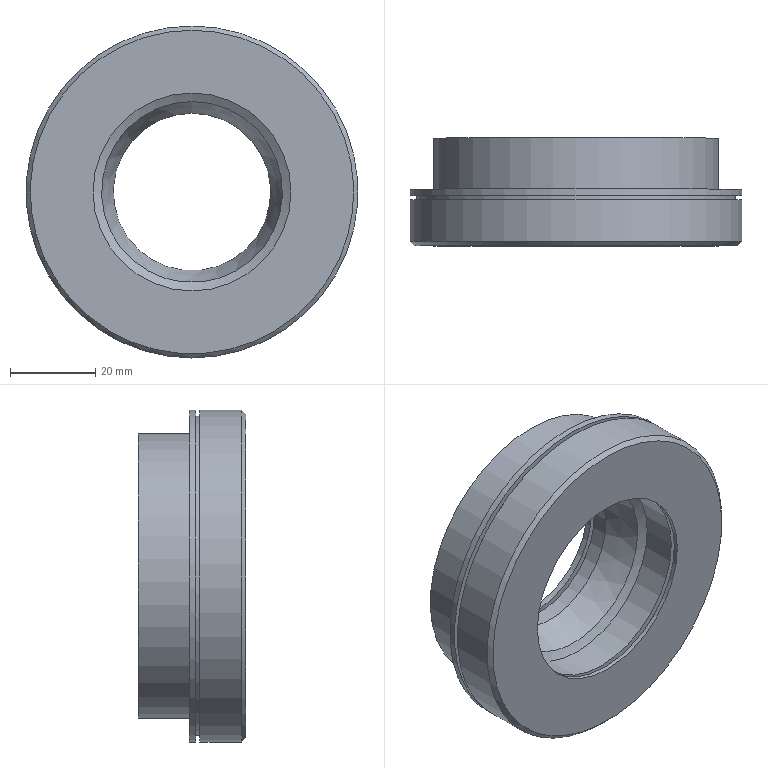Part | STEP file | Inner part of clamp | 1 solid | 38 faces | box 78 x 25.32 x 78 mm | volume 67715 mm3 | cylinder 14 | plane 13 | cone 7 | torus 4 | commonest cylinder face diameters 8 x4 37 x2 46.5 x2 78 x2 40 x1 49.5 x1
STEP:
#1=CARTESIAN_POINT('',(0.,-14.5,39.));
#2=VERTEX_POINT('',#1);
#3=CARTESIAN_POINT('',(0.,-14.5,0.));
#4=DIRECTION('',(0.,1.,0.));
#5=DIRECTION('',(0.,0.,1.));
#6=AXIS2_PLACEMENT_3D('',#3,#4,#5);
#7=CIRCLE('',#6,39.);
#8=EDGE_CURVE('',#2,#2,#7,.F.);
#9=ORIENTED_EDGE('',*,*,#8,.T.);
#10=EDGE_LOOP('',(#9));
#11=FACE_OUTER_BOUND('',#10,.T.);
#12=CARTESIAN_POINT('',(0.,-24.32,39.));
#13=VERTEX_POINT('',#12);
#14=CARTESIAN_POINT('',(0.,-24.32,0.));
#15=DIRECTION('',(0.,1.,0.));
#16=DIRECTION('',(0.,0.,1.));
#17=AXIS2_PLACEMENT_3D('',#14,#15,#16);
#18=CIRCLE('',#17,39.);
#19=EDGE_CURVE('',#13,#13,#18,.T.);
#20=ORIENTED_EDGE('',*,*,#19,.T.);
#21=EDGE_LOOP('',(#20));
#22=FACE_OUTER_BOUND('',#21,.T.);
#23=CARTESIAN_POINT('',(0.,-22.,0.));
#24=DIRECTION('',(0.,1.,0.));
#25=DIRECTION('',(0.,0.,1.));
#26=AXIS2_PLACEMENT_3D('',#23,#24,#25);
#27=CYLINDRICAL_SURFACE('',#26,39.);
#28=ADVANCED_FACE('',(#11,#22),#27,.T.);
#29=CARTESIAN_POINT('',(0.,-25.32,38.));
#30=VERTEX_POINT('',#29);
#31=CARTESIAN_POINT('',(0.,-25.32,0.));
#32=DIRECTION('',(0.,1.,0.));
#33=DIRECTION('',(0.,0.,1.));
#34=AXIS2_PLACEMENT_3D('',#31,#32,#33);
#35=CIRCLE('',#34,38.);
#36=EDGE_CURVE('',#30,#30,#35,.T.);
#37=ORIENTED_EDGE('',*,*,#36,.F.);
#38=EDGE_LOOP('',(#37));
#39=FACE_BOUND('',#38,.T.);
#40=CARTESIAN_POINT('',(0.,-25.32,23.25));
#41=VERTEX_POINT('',#40);
#42=CARTESIAN_POINT('',(0.,-25.32,0.));
#43=DIRECTION('',(0.,1.,0.));
#44=DIRECTION('',(0.,0.,1.));
#45=AXIS2_PLACEMENT_3D('',#42,#43,#44);
#46=CIRCLE('',#45,23.25);
#47=EDGE_CURVE('',#41,#41,#46,.T.);
#48=ORIENTED_EDGE('',*,*,#47,.T.);
#49=EDGE_LOOP('',(#48));
#50=FACE_BOUND('',#49,.T.);
#51=CARTESIAN_POINT('',(0.,-25.32,0.));
#52=DIRECTION('',(0.,-1.,0.));
#53=DIRECTION('',(0.,0.,1.));
#54=AXIS2_PLACEMENT_3D('',#51,#52,#53);
#55=PLANE('',#54);
#56=ADVANCED_FACE('',(#39,#50),#55,.T.);
#57=ORIENTED_EDGE('',*,*,#8,.F.);
#58=EDGE_LOOP('',(#57));
#59=FACE_BOUND('',#58,.T.);
#60=CARTESIAN_POINT('',(0.,-14.5,37.5));
#61=VERTEX_POINT('',#60);
#62=CARTESIAN_POINT('',(0.,-14.5,0.));
#63=DIRECTION('',(0.,1.,0.));
#64=DIRECTION('',(0.,0.,1.));
#65=AXIS2_PLACEMENT_3D('',#62,#63,#64);
#66=CIRCLE('',#65,37.5);
#67=EDGE_CURVE('',#61,#61,#66,.T.);
#68=ORIENTED_EDGE('',*,*,#67,.F.);
#69=EDGE_LOOP('',(#68));
#70=FACE_BOUND('',#69,.T.);
#71=CARTESIAN_POINT('',(0.,-14.5,0.));
#72=DIRECTION('',(0.,-1.,0.));
#73=DIRECTION('',(0.,0.,1.));
#74=AXIS2_PLACEMENT_3D('',#71,#72,#73);
#75=PLANE('',#74);
#76=ADVANCED_FACE('',(#59,#70),#75,.F.);
#77=CARTESIAN_POINT('',(0.,-24.32,23.25));
#78=VERTEX_POINT('',#77);
#79=CARTESIAN_POINT('',(0.,-24.32,0.));
#80=DIRECTION('',(0.,1.,0.));
#81=DIRECTION('',(0.,0.,1.));
#82=AXIS2_PLACEMENT_3D('',#79,#80,#81);
#83=CIRCLE('',#82,23.25);
#84=EDGE_CURVE('',#78,#78,#83,.T.);
#85=ORIENTED_EDGE('',*,*,#84,.T.);
#86=EDGE_LOOP('',(#85));
#87=FACE_OUTER_BOUND('',#86,.T.);
#88=ORIENTED_EDGE('',*,*,#47,.F.);
#89=EDGE_LOOP('',(#88));
#90=FACE_OUTER_BOUND('',#89,.T.);
#91=CARTESIAN_POINT('',(0.,-15.32,0.));
#92=DIRECTION('',(0.,1.,0.));
#93=DIRECTION('',(0.,0.,1.));
#94=AXIS2_PLACEMENT_3D('',#91,#92,#93);
#95=CYLINDRICAL_SURFACE('',#94,23.25);
#96=ADVANCED_FACE('',(#87,#90),#95,.F.);
#97=CARTESIAN_POINT('',(0.,-13.5,37.5));
#98=VERTEX_POINT('',#97);
#99=CARTESIAN_POINT('',(0.,-13.5,0.));
#100=DIRECTION('',(0.,1.,0.));
#101=DIRECTION('',(0.,0.,1.));
#102=AXIS2_PLACEMENT_3D('',#99,#100,#101);
#103=CIRCLE('',#102,37.5);
#104=EDGE_CURVE('',#98,#98,#103,.T.);
#105=ORIENTED_EDGE('',*,*,#104,.F.);
#106=EDGE_LOOP('',(#105));
#107=FACE_OUTER_BOUND('',#106,.T.);
#108=ORIENTED_EDGE('',*,*,#67,.T.);
#109=EDGE_LOOP('',(#108));
#110=FACE_OUTER_BOUND('',#109,.T.);
#111=CARTESIAN_POINT('',(0.,-13.5,0.));
#112=DIRECTION('',(0.,1.,0.));
#113=DIRECTION('',(0.,0.,1.));
#114=AXIS2_PLACEMENT_3D('',#111,#112,#113);
#115=CYLINDRICAL_SURFACE('',#114,37.5);
#116=ADVANCED_FACE('',(#107,#110),#115,.T.);
#117=CARTESIAN_POINT('',(0.,-24.32,24.75));
#118=VERTEX_POINT('',#117);
#119=CARTESIAN_POINT('',(0.,-24.32,0.));
#120=DIRECTION('',(0.,1.,0.));
#121=DIRECTION('',(0.,0.,1.));
#122=AXIS2_PLACEMENT_3D('',#119,#120,#121);
#123=CIRCLE('',#122,24.75);
#124=EDGE_CURVE('',#118,#118,#123,.T.);
#125=ORIENTED_EDGE('',*,*,#124,.T.);
#126=EDGE_LOOP('',(#125));
#127=FACE_BOUND('',#126,.T.);
#128=ORIENTED_EDGE('',*,*,#84,.F.);
#129=EDGE_LOOP('',(#128));
#130=FACE_BOUND('',#129,.T.);
#131=CARTESIAN_POINT('',(0.,-24.32,0.));
#132=DIRECTION('',(0.,-1.,0.));
#133=DIRECTION('',(0.,0.,1.));
#134=AXIS2_PLACEMENT_3D('',#131,#132,#133);
#135=PLANE('',#134);
#136=ADVANCED_FACE('',(#127,#130),#135,.F.);
#137=CARTESIAN_POINT('',(0.,-13.5,39.));
#138=VERTEX_POINT('',#137);
#139=CARTESIAN_POINT('',(0.,-13.5,0.));
#140=DIRECTION('',(0.,1.,0.));
#141=DIRECTION('',(0.,0.,1.));
#142=AXIS2_PLACEMENT_3D('',#139,#140,#141);
#143=CIRCLE('',#142,39.);
#144=EDGE_CURVE('',#138,#138,#143,.T.);
#145=ORIENTED_EDGE('',*,*,#144,.F.);
#146=EDGE_LOOP('',(#145));
#147=FACE_BOUND('',#146,.T.);
#148=ORIENTED_EDGE('',*,*,#104,.T.);
#149=EDGE_LOOP('',(#148));
#150=FACE_BOUND('',#149,.T.);
#151=CARTESIAN_POINT('',(0.,-13.5,0.));
#152=DIRECTION('',(0.,1.,0.));
#153=DIRECTION('',(0.,0.,1.));
#154=AXIS2_PLACEMENT_3D('',#151,#152,#153);
#155=PLANE('',#154);
#156=ADVANCED_FACE('',(#147,#150),#155,.F.);
#157=CARTESIAN_POINT('',(0.,-23.32,24.75));
#158=VERTEX_POINT('',#157);
#159=CARTESIAN_POINT('',(0.,-23.32,0.));
#160=DIRECTION('',(0.,1.,0.));
#161=DIRECTION('',(0.,0.,1.));
#162=AXIS2_PLACEMENT_3D('',#159,#160,#161);
#163=CIRCLE('',#162,24.75);
#164=EDGE_CURVE('',#158,#158,#163,.T.);
#165=ORIENTED_EDGE('',*,*,#164,.T.);
#166=EDGE_LOOP('',(#165));
#167=FACE_OUTER_BOUND('',#166,.T.);
#168=ORIENTED_EDGE('',*,*,#124,.F.);
#169=EDGE_LOOP('',(#168));
#170=FACE_OUTER_BOUND('',#169,.T.);
#171=CARTESIAN_POINT('',(0.,-24.32,0.));
#172=DIRECTION('',(0.,1.,0.));
#173=DIRECTION('',(0.,0.,1.));
#174=AXIS2_PLACEMENT_3D('',#171,#172,#173);
#175=CYLINDRICAL_SURFACE('',#174,24.75);
#176=ADVANCED_FACE('',(#167,#170),#175,.F.);
#177=CARTESIAN_POINT('',(0.,-12.,39.));
#178=VERTEX_POINT('',#177);
#179=CARTESIAN_POINT('',(0.,-12.,0.));
#180=DIRECTION('',(0.,1.,0.));
#181=DIRECTION('',(0.,0.,1.));
#182=AXIS2_PLACEMENT_3D('',#179,#180,#181);
#183=CIRCLE('',#182,39.);
#184=EDGE_CURVE('',#178,#178,#183,.T.);
#185=ORIENTED_EDGE('',*,*,#184,.F.);
#186=EDGE_LOOP('',(#185));
#187=FACE_OUTER_BOUND('',#186,.T.);
#188=ORIENTED_EDGE('',*,*,#144,.T.);
#189=EDGE_LOOP('',(#188));
#190=FACE_OUTER_BOUND('',#189,.T.);
#191=CARTESIAN_POINT('',(0.,-22.,0.));
#192=DIRECTION('',(0.,1.,0.));
#193=DIRECTION('',(0.,0.,1.));
#194=AXIS2_PLACEMENT_3D('',#191,#192,#193);
#195=CYLINDRICAL_SURFACE('',#194,39.);
#196=ADVANCED_FACE('',(#187,#190),#195,.T.);
#197=ORIENTED_EDGE('',*,*,#164,.F.);
#198=EDGE_LOOP('',(#197));
#199=FACE_BOUND('',#198,.T.);
#200=CARTESIAN_POINT('',(0.,-23.32,23.25));
#201=VERTEX_POINT('',#200);
#202=CARTESIAN_POINT('',(0.,-23.32,0.));
#203=DIRECTION('',(0.,1.,0.));
#204=DIRECTION('',(0.,0.,1.));
#205=AXIS2_PLACEMENT_3D('',#202,#203,#204);
#206=CIRCLE('',#205,23.25);
#207=EDGE_CURVE('',#201,#201,#206,.F.);
#208=ORIENTED_EDGE('',*,*,#207,.F.);
#209=EDGE_LOOP('',(#208));
#210=FACE_BOUND('',#209,.T.);
#211=CARTESIAN_POINT('',(0.,-23.32,0.));
#212=DIRECTION('',(0.,1.,0.));
#213=DIRECTION('',(0.,0.,1.));
#214=AXIS2_PLACEMENT_3D('',#211,#212,#213);
#215=PLANE('',#214);
#216=ADVANCED_FACE('',(#199,#210),#215,.F.);
#217=ORIENTED_EDGE('',*,*,#184,.T.);
#218=EDGE_LOOP('',(#217));
#219=FACE_BOUND('',#218,.T.);
#220=CARTESIAN_POINT('',(0.,-12.,33.5));
#221=VERTEX_POINT('',#220);
#222=CARTESIAN_POINT('',(0.,-12.,0.));
#223=DIRECTION('',(0.,1.,0.));
#224=DIRECTION('',(0.,0.,1.));
#225=AXIS2_PLACEMENT_3D('',#222,#223,#224);
#226=CIRCLE('',#225,33.5);
#227=EDGE_CURVE('',#221,#221,#226,.T.);
#228=ORIENTED_EDGE('',*,*,#227,.F.);
#229=EDGE_LOOP('',(#228));
#230=FACE_BOUND('',#229,.T.);
#231=CARTESIAN_POINT('',(0.,-12.,0.));
#232=DIRECTION('',(0.,1.,0.));
#233=DIRECTION('',(0.,0.,1.));
#234=AXIS2_PLACEMENT_3D('',#231,#232,#233);
#235=PLANE('',#234);
#236=ADVANCED_FACE('',(#219,#230),#235,.T.);
#237=CARTESIAN_POINT('',(0.,-15.32,23.25));
#238=VERTEX_POINT('',#237);
#239=CARTESIAN_POINT('',(0.,-15.32,0.));
#240=DIRECTION('',(0.,1.,0.));
#241=DIRECTION('',(0.,0.,1.));
#242=AXIS2_PLACEMENT_3D('',#239,#240,#241);
#243=CIRCLE('',#242,23.25);
#244=EDGE_CURVE('',#238,#238,#243,.T.);
#245=ORIENTED_EDGE('',*,*,#244,.T.);
#246=EDGE_LOOP('',(#245));
#247=FACE_OUTER_BOUND('',#246,.T.);
#248=ORIENTED_EDGE('',*,*,#207,.T.);
#249=EDGE_LOOP('',(#248));
#250=FACE_OUTER_BOUND('',#249,.T.);
#251=CARTESIAN_POINT('',(0.,-15.32,0.));
#252=DIRECTION('',(0.,1.,0.));
#253=DIRECTION('',(0.,0.,1.));
#254=AXIS2_PLACEMENT_3D('',#251,#252,#253);
#255=CYLINDRICAL_SURFACE('',#254,23.25);
#256=ADVANCED_FACE('',(#247,#250),#255,.F.);
#257=CARTESIAN_POINT('',(0.,0.,33.5));
#258=VERTEX_POINT('',#257);
#259=CARTESIAN_POINT('',(0.,0.,0.));
#260=DIRECTION('',(0.,1.,0.));
#261=DIRECTION('',(0.,0.,1.));
#262=AXIS2_PLACEMENT_3D('',#259,#260,#261);
#263=CIRCLE('',#262,33.5);
#264=EDGE_CURVE('',#258,#258,#263,.T.);
#265=ORIENTED_EDGE('',*,*,#264,.F.);
#266=EDGE_LOOP('',(#265));
#267=FACE_OUTER_BOUND('',#266,.T.);
#268=ORIENTED_EDGE('',*,*,#227,.T.);
#269=EDGE_LOOP('',(#268));
#270=FACE_OUTER_BOUND('',#269,.T.);
#271=CARTESIAN_POINT('',(0.,-12.,0.));
#272=DIRECTION('',(0.,1.,0.));
#273=DIRECTION('',(0.,0.,1.));
#274=AXIS2_PLACEMENT_3D('',#271,#272,#273);
#275=CYLINDRICAL_SURFACE('',#274,33.5);
#276=ADVANCED_FACE('',(#267,#270),#275,.T.);
#277=CARTESIAN_POINT('',(0.,-14.165,21.25));
#278=VERTEX_POINT('',#277);
#279=CARTESIAN_POINT('',(0.,-14.165,0.));
#280=DIRECTION('',(0.,1.,0.));
#281=DIRECTION('',(0.,0.,1.));
#282=AXIS2_PLACEMENT_3D('',#279,#280,#281);
#283=CIRCLE('',#282,21.25);
#284=EDGE_CURVE('',#278,#278,#283,.T.);
#285=ORIENTED_EDGE('',*,*,#284,.T.);
#286=EDGE_LOOP('',(#285));
#287=FACE_OUTER_BOUND('',#286,.T.);
#288=ORIENTED_EDGE('',*,*,#244,.F.);
#289=EDGE_LOOP('',(#288));
#290=FACE_OUTER_BOUND('',#289,.T.);
#291=CARTESIAN_POINT('',(0.,-14.742,0.));
#292=DIRECTION('',(0.,-1.,0.));
#293=DIRECTION('',(0.,0.,-1.));
#294=AXIS2_PLACEMENT_3D('',#291,#292,#293);
#295=CONICAL_SURFACE('',#294,22.25,1.047);
#296=ADVANCED_FACE('',(#287,#290),#295,.F.);
#297=ORIENTED_EDGE('',*,*,#264,.T.);
#298=EDGE_LOOP('',(#297));
#299=FACE_BOUND('',#298,.T.);
#300=CARTESIAN_POINT('',(23.,0.,0.));
#301=VERTEX_POINT('',#300);
#302=CARTESIAN_POINT('',(27.5,0.,0.));
#303=DIRECTION('',(0.,1.,0.));
#304=DIRECTION('',(-1.,0.,0.));
#305=AXIS2_PLACEMENT_3D('',#302,#303,#304);
#306=CIRCLE('',#305,4.5);
#307=EDGE_CURVE('',#301,#301,#306,.F.);
#308=ORIENTED_EDGE('',*,*,#307,.T.);
#309=EDGE_LOOP('',(#308));
#310=FACE_BOUND('',#309,.T.);
#311=CARTESIAN_POINT('',(-23.,0.,0.));
#312=VERTEX_POINT('',#311);
#313=CARTESIAN_POINT('',(-27.5,0.,0.));
#314=DIRECTION('',(0.,1.,0.));
#315=DIRECTION('',(1.,0.,0.));
#316=AXIS2_PLACEMENT_3D('',#313,#314,#315);
#317=CIRCLE('',#316,4.5);
#318=EDGE_CURVE('',#312,#312,#317,.F.);
#319=ORIENTED_EDGE('',*,*,#318,.T.);
#320=EDGE_LOOP('',(#319));
#321=FACE_BOUND('',#320,.T.);
#322=CARTESIAN_POINT('',(0.,0.,23.));
#323=VERTEX_POINT('',#322);
#324=CARTESIAN_POINT('',(0.,0.,27.5));
#325=DIRECTION('',(0.,1.,0.));
#326=DIRECTION('',(0.,0.,-1.));
#327=AXIS2_PLACEMENT_3D('',#324,#325,#326);
#328=CIRCLE('',#327,4.5);
#329=EDGE_CURVE('',#323,#323,#328,.F.);
#330=ORIENTED_EDGE('',*,*,#329,.T.);
#331=EDGE_LOOP('',(#330));
#332=FACE_BOUND('',#331,.T.);
#333=CARTESIAN_POINT('',(0.,0.,18.5));
#334=VERTEX_POINT('',#333);
#335=CARTESIAN_POINT('',(0.,0.,0.));
#336=DIRECTION('',(0.,1.,0.));
#337=DIRECTION('',(0.,0.,1.));
#338=AXIS2_PLACEMENT_3D('',#335,#336,#337);
#339=CIRCLE('',#338,18.5);
#340=EDGE_CURVE('',#334,#334,#339,.T.);
#341=ORIENTED_EDGE('',*,*,#340,.F.);
#342=EDGE_LOOP('',(#341));
#343=FACE_BOUND('',#342,.T.);
#344=CARTESIAN_POINT('',(0.,0.,-23.));
#345=VERTEX_POINT('',#344);
#346=CARTESIAN_POINT('',(0.,0.,-27.5));
#347=DIRECTION('',(0.,1.,0.));
#348=DIRECTION('',(0.,0.,1.));
#349=AXIS2_PLACEMENT_3D('',#346,#347,#348);
#350=CIRCLE('',#349,4.5);
#351=EDGE_CURVE('',#345,#345,#350,.F.);
#352=ORIENTED_EDGE('',*,*,#351,.T.);
#353=EDGE_LOOP('',(#352));
#354=FACE_BOUND('',#353,.T.);
#355=CARTESIAN_POINT('',(0.,0.,0.));
#356=DIRECTION('',(0.,1.,0.));
#357=DIRECTION('',(0.,0.,1.));
#358=AXIS2_PLACEMENT_3D('',#355,#356,#357);
#359=PLANE('',#358);
#360=ADVANCED_FACE('',(#299,#310,#321,#332,#343,#354),#359,.T.);
#361=CARTESIAN_POINT('',(0.,-6.289,18.5));
#362=VERTEX_POINT('',#361);
#363=CARTESIAN_POINT('',(0.,-6.289,0.));
#364=DIRECTION('',(0.,1.,0.));
#365=DIRECTION('',(0.,0.,1.));
#366=AXIS2_PLACEMENT_3D('',#363,#364,#365);
#367=CIRCLE('',#366,18.5);
#368=EDGE_CURVE('',#362,#362,#367,.T.);
#369=ORIENTED_EDGE('',*,*,#368,.T.);
#370=EDGE_LOOP('',(#369));
#371=FACE_OUTER_BOUND('',#370,.T.);
#372=ORIENTED_EDGE('',*,*,#284,.F.);
#373=EDGE_LOOP('',(#372));
#374=FACE_OUTER_BOUND('',#373,.T.);
#375=CARTESIAN_POINT('',(0.,-10.227,0.));
#376=DIRECTION('',(0.,-1.,0.));
#377=DIRECTION('',(0.,0.,-1.));
#378=AXIS2_PLACEMENT_3D('',#375,#376,#377);
#379=CONICAL_SURFACE('',#378,19.875,0.3359);
#380=ADVANCED_FACE('',(#371,#374),#379,.F.);
#381=CARTESIAN_POINT('',(23.5,-0.5,0.));
#382=VERTEX_POINT('',#381);
#383=CARTESIAN_POINT('',(27.5,-0.5,0.));
#384=DIRECTION('',(0.,1.,0.));
#385=DIRECTION('',(-1.,0.,0.));
#386=AXIS2_PLACEMENT_3D('',#383,#384,#385);
#387=CIRCLE('',#386,4.);
#388=EDGE_CURVE('',#382,#382,#387,.F.);
#389=ORIENTED_EDGE('',*,*,#388,.T.);
#390=EDGE_LOOP('',(#389));
#391=FACE_OUTER_BOUND('',#390,.T.);
#392=ORIENTED_EDGE('',*,*,#307,.F.);
#393=EDGE_LOOP('',(#392));
#394=FACE_OUTER_BOUND('',#393,.T.);
#395=CARTESIAN_POINT('',(27.5,-0.25,0.));
#396=DIRECTION('',(0.,1.,0.));
#397=DIRECTION('',(-1.,0.,0.));
#398=AXIS2_PLACEMENT_3D('',#395,#396,#397);
#399=CONICAL_SURFACE('',#398,4.25,0.7854);
#400=ADVANCED_FACE('',(#391,#394),#399,.F.);
#401=ORIENTED_EDGE('',*,*,#318,.F.);
#402=EDGE_LOOP('',(#401));
#403=FACE_OUTER_BOUND('',#402,.T.);
#404=CARTESIAN_POINT('',(-23.5,-0.5,0.));
#405=VERTEX_POINT('',#404);
#406=CARTESIAN_POINT('',(-27.5,-0.5,0.));
#407=DIRECTION('',(0.,1.,0.));
#408=DIRECTION('',(1.,0.,0.));
#409=AXIS2_PLACEMENT_3D('',#406,#407,#408);
#410=CIRCLE('',#409,4.);
#411=EDGE_CURVE('',#405,#405,#410,.F.);
#412=ORIENTED_EDGE('',*,*,#411,.T.);
#413=EDGE_LOOP('',(#412));
#414=FACE_OUTER_BOUND('',#413,.T.);
#415=CARTESIAN_POINT('',(-27.5,-0.25,0.));
#416=DIRECTION('',(0.,1.,0.));
#417=DIRECTION('',(1.,0.,0.));
#418=AXIS2_PLACEMENT_3D('',#415,#416,#417);
#419=CONICAL_SURFACE('',#418,4.25,0.7854);
#420=ADVANCED_FACE('',(#403,#414),#419,.F.);
#421=ORIENTED_EDGE('',*,*,#329,.F.);
#422=EDGE_LOOP('',(#421));
#423=FACE_OUTER_BOUND('',#422,.T.);
#424=CARTESIAN_POINT('',(0.,-0.5,23.5));
#425=VERTEX_POINT('',#424);
#426=CARTESIAN_POINT('',(0.,-0.5,27.5));
#427=DIRECTION('',(0.,1.,0.));
#428=DIRECTION('',(0.,0.,-1.));
#429=AXIS2_PLACEMENT_3D('',#426,#427,#428);
#430=CIRCLE('',#429,4.);
#431=EDGE_CURVE('',#425,#425,#430,.F.);
#432=ORIENTED_EDGE('',*,*,#431,.T.);
#433=EDGE_LOOP('',(#432));
#434=FACE_OUTER_BOUND('',#433,.T.);
#435=CARTESIAN_POINT('',(0.,-0.25,27.5));
#436=DIRECTION('',(0.,1.,0.));
#437=DIRECTION('',(0.,0.,-1.));
#438=AXIS2_PLACEMENT_3D('',#435,#436,#437);
#439=CONICAL_SURFACE('',#438,4.25,0.7854);
#440=ADVANCED_FACE('',(#423,#434),#439,.F.);
#441=ORIENTED_EDGE('',*,*,#340,.T.);
#442=EDGE_LOOP('',(#441));
#443=FACE_OUTER_BOUND('',#442,.T.);
#444=CARTESIAN_POINT('',(0.,-1.5,18.5));
#445=VERTEX_POINT('',#444);
#446=CARTESIAN_POINT('',(0.,-1.5,0.));
#447=DIRECTION('',(0.,1.,0.));
#448=DIRECTION('',(0.,0.,1.));
#449=AXIS2_PLACEMENT_3D('',#446,#447,#448);
#450=CIRCLE('',#449,18.5);
#451=EDGE_CURVE('',#445,#445,#450,.F.);
#452=ORIENTED_EDGE('',*,*,#451,.T.);
#453=EDGE_LOOP('',(#452));
#454=FACE_OUTER_BOUND('',#453,.T.);
#455=CARTESIAN_POINT('',(0.,0.,0.));
#456=DIRECTION('',(0.,1.,0.));
#457=DIRECTION('',(0.,0.,1.));
#458=AXIS2_PLACEMENT_3D('',#455,#456,#457);
#459=CYLINDRICAL_SURFACE('',#458,18.5);
#460=ADVANCED_FACE('',(#443,#454),#459,.F.);
#461=ORIENTED_EDGE('',*,*,#351,.F.);
#462=EDGE_LOOP('',(#461));
#463=FACE_OUTER_BOUND('',#462,.T.);
#464=CARTESIAN_POINT('',(0.,-0.5,-23.5));
#465=VERTEX_POINT('',#464);
#466=CARTESIAN_POINT('',(0.,-0.5,-27.5));
#467=DIRECTION('',(0.,1.,0.));
#468=DIRECTION('',(0.,0.,1.));
#469=AXIS2_PLACEMENT_3D('',#466,#467,#468);
#470=CIRCLE('',#469,4.);
#471=EDGE_CURVE('',#465,#465,#470,.F.);
#472=ORIENTED_EDGE('',*,*,#471,.T.);
#473=EDGE_LOOP('',(#472));
#474=FACE_OUTER_BOUND('',#473,.T.);
#475=CARTESIAN_POINT('',(0.,-0.25,-27.5));
#476=DIRECTION('',(0.,1.,0.));
#477=DIRECTION('',(0.,0.,1.));
#478=AXIS2_PLACEMENT_3D('',#475,#476,#477);
#479=CONICAL_SURFACE('',#478,4.25,0.7854);
#480=ADVANCED_FACE('',(#463,#474),#479,.F.);
#481=CARTESIAN_POINT('',(0.,-2.5,18.5));
#482=VERTEX_POINT('',#481);
#483=CARTESIAN_POINT('',(0.,-2.5,0.));
#484=DIRECTION('',(0.,1.,0.));
#485=DIRECTION('',(0.,0.,1.));
#486=AXIS2_PLACEMENT_3D('',#483,#484,#485);
#487=CIRCLE('',#486,18.5);
#488=EDGE_CURVE('',#482,#482,#487,.T.);
#489=ORIENTED_EDGE('',*,*,#488,.T.);
#490=EDGE_LOOP('',(#489));
#491=FACE_OUTER_BOUND('',#490,.T.);
#492=ORIENTED_EDGE('',*,*,#368,.F.);
#493=EDGE_LOOP('',(#492));
#494=FACE_OUTER_BOUND('',#493,.T.);
#495=CARTESIAN_POINT('',(0.,0.,0.));
#496=DIRECTION('',(0.,1.,0.));
#497=DIRECTION('',(0.,0.,1.));
#498=AXIS2_PLACEMENT_3D('',#495,#496,#497);
#499=CYLINDRICAL_SURFACE('',#498,18.5);
#500=ADVANCED_FACE('',(#491,#494),#499,.F.);
#501=ORIENTED_EDGE('',*,*,#388,.F.);
#502=EDGE_LOOP('',(#501));
#503=FACE_OUTER_BOUND('',#502,.T.);
#504=CARTESIAN_POINT('',(23.5,-9.5,0.));
#505=VERTEX_POINT('',#504);
#506=CARTESIAN_POINT('',(27.5,-9.5,0.));
#507=DIRECTION('',(0.,1.,0.));
#508=DIRECTION('',(-1.,0.,0.));
#509=AXIS2_PLACEMENT_3D('',#506,#507,#508);
#510=CIRCLE('',#509,4.);
#511=EDGE_CURVE('',#505,#505,#510,.T.);
#512=ORIENTED_EDGE('',*,*,#511,.F.);
#513=EDGE_LOOP('',(#512));
#514=FACE_OUTER_BOUND('',#513,.T.);
#515=CARTESIAN_POINT('',(27.5,-10.,0.));
#516=DIRECTION('',(0.,1.,0.));
#517=DIRECTION('',(-1.,0.,0.));
#518=AXIS2_PLACEMENT_3D('',#515,#516,#517);
#519=CYLINDRICAL_SURFACE('',#518,4.);
#520=ADVANCED_FACE('',(#503,#514),#519,.F.);
#521=ORIENTED_EDGE('',*,*,#411,.F.);
#522=EDGE_LOOP('',(#521));
#523=FACE_OUTER_BOUND('',#522,.T.);
#524=CARTESIAN_POINT('',(-23.5,-9.5,0.));
#525=VERTEX_POINT('',#524);
#526=CARTESIAN_POINT('',(-27.5,-9.5,0.));
#527=DIRECTION('',(0.,1.,0.));
#528=DIRECTION('',(1.,0.,0.));
#529=AXIS2_PLACEMENT_3D('',#526,#527,#528);
#530=CIRCLE('',#529,4.);
#531=EDGE_CURVE('',#525,#525,#530,.T.);
#532=ORIENTED_EDGE('',*,*,#531,.F.);
#533=EDGE_LOOP('',(#532));
#534=FACE_OUTER_BOUND('',#533,.T.);
#535=CARTESIAN_POINT('',(-27.5,-10.,0.));
#536=DIRECTION('',(0.,1.,0.));
#537=DIRECTION('',(1.,0.,0.));
#538=AXIS2_PLACEMENT_3D('',#535,#536,#537);
#539=CYLINDRICAL_SURFACE('',#538,4.);
#540=ADVANCED_FACE('',(#523,#534),#539,.F.);
#541=ORIENTED_EDGE('',*,*,#431,.F.);
#542=EDGE_LOOP('',(#541));
#543=FACE_OUTER_BOUND('',#542,.T.);
#544=CARTESIAN_POINT('',(0.,-9.5,23.5));
#545=VERTEX_POINT('',#544);
#546=CARTESIAN_POINT('',(0.,-9.5,27.5));
#547=DIRECTION('',(0.,1.,0.));
#548=DIRECTION('',(0.,0.,-1.));
#549=AXIS2_PLACEMENT_3D('',#546,#547,#548);
#550=CIRCLE('',#549,4.);
#551=EDGE_CURVE('',#545,#545,#550,.T.);
#552=ORIENTED_EDGE('',*,*,#551,.F.);
#553=EDGE_LOOP('',(#552));
#554=FACE_OUTER_BOUND('',#553,.T.);
#555=CARTESIAN_POINT('',(0.,-10.,27.5));
#556=DIRECTION('',(0.,1.,0.));
#557=DIRECTION('',(0.,0.,-1.));
#558=AXIS2_PLACEMENT_3D('',#555,#556,#557);
#559=CYLINDRICAL_SURFACE('',#558,4.);
#560=ADVANCED_FACE('',(#543,#554),#559,.F.);
#561=CARTESIAN_POINT('',(0.,-1.5,20.));
#562=VERTEX_POINT('',#561);
#563=CARTESIAN_POINT('',(0.,-1.5,0.));
#564=DIRECTION('',(0.,1.,0.));
#565=DIRECTION('',(0.,0.,1.));
#566=AXIS2_PLACEMENT_3D('',#563,#564,#565);
#567=CIRCLE('',#566,20.);
#568=EDGE_CURVE('',#562,#562,#567,.T.);
#569=ORIENTED_EDGE('',*,*,#568,.F.);
#570=EDGE_LOOP('',(#569));
#571=FACE_BOUND('',#570,.T.);
#572=ORIENTED_EDGE('',*,*,#451,.F.);
#573=EDGE_LOOP('',(#572));
#574=FACE_BOUND('',#573,.T.);
#575=CARTESIAN_POINT('',(0.,-1.5,0.));
#576=DIRECTION('',(0.,1.,0.));
#577=DIRECTION('',(0.,0.,1.));
#578=AXIS2_PLACEMENT_3D('',#575,#576,#577);
#579=PLANE('',#578);
#580=ADVANCED_FACE('',(#571,#574),#579,.F.);
#581=ORIENTED_EDGE('',*,*,#471,.F.);
#582=EDGE_LOOP('',(#581));
#583=FACE_OUTER_BOUND('',#582,.T.);
#584=CARTESIAN_POINT('',(0.,-9.5,-23.5));
#585=VERTEX_POINT('',#584);
#586=CARTESIAN_POINT('',(0.,-9.5,-27.5));
#587=DIRECTION('',(0.,1.,0.));
#588=DIRECTION('',(0.,0.,1.));
#589=AXIS2_PLACEMENT_3D('',#586,#587,#588);
#590=CIRCLE('',#589,4.);
#591=EDGE_CURVE('',#585,#585,#590,.T.);
#592=ORIENTED_EDGE('',*,*,#591,.F.);
#593=EDGE_LOOP('',(#592));
#594=FACE_OUTER_BOUND('',#593,.T.);
#595=CARTESIAN_POINT('',(0.,-10.,-27.5));
#596=DIRECTION('',(0.,1.,0.));
#597=DIRECTION('',(0.,0.,1.));
#598=AXIS2_PLACEMENT_3D('',#595,#596,#597);
#599=CYLINDRICAL_SURFACE('',#598,4.);
#600=ADVANCED_FACE('',(#583,#594),#599,.F.);
#601=CARTESIAN_POINT('',(0.,-2.5,20.));
#602=VERTEX_POINT('',#601);
#603=CARTESIAN_POINT('',(0.,-2.5,0.));
#604=DIRECTION('',(0.,1.,0.));
#605=DIRECTION('',(0.,0.,1.));
#606=AXIS2_PLACEMENT_3D('',#603,#604,#605);
#607=CIRCLE('',#606,20.);
#608=EDGE_CURVE('',#602,#602,#607,.T.);
#609=ORIENTED_EDGE('',*,*,#608,.T.);
#610=EDGE_LOOP('',(#609));
#611=FACE_BOUND('',#610,.T.);
#612=ORIENTED_EDGE('',*,*,#488,.F.);
#613=EDGE_LOOP('',(#612));
#614=FACE_BOUND('',#613,.T.);
#615=CARTESIAN_POINT('',(0.,-2.5,0.));
#616=DIRECTION('',(0.,-1.,0.));
#617=DIRECTION('',(0.,0.,1.));
#618=AXIS2_PLACEMENT_3D('',#615,#616,#617);
#619=PLANE('',#618);
#620=ADVANCED_FACE('',(#611,#614),#619,.F.);
#621=CARTESIAN_POINT('',(24.,-10.,0.));
#622=VERTEX_POINT('',#621);
#623=CARTESIAN_POINT('',(27.5,-10.,0.));
#624=DIRECTION('',(0.,1.,0.));
#625=DIRECTION('',(-1.,0.,0.));
#626=AXIS2_PLACEMENT_3D('',#623,#624,#625);
#627=CIRCLE('',#626,3.5);
#628=EDGE_CURVE('',#622,#622,#627,.T.);
#629=ORIENTED_EDGE('',*,*,#628,.F.);
#630=EDGE_LOOP('',(#629));
#631=FACE_OUTER_BOUND('',#630,.T.);
#632=ORIENTED_EDGE('',*,*,#511,.T.);
#633=EDGE_LOOP('',(#632));
#634=FACE_OUTER_BOUND('',#633,.T.);
#635=CARTESIAN_POINT('',(27.5,-9.5,0.));
#636=DIRECTION('',(0.,1.,0.));
#637=DIRECTION('',(-1.,0.,0.));
#638=AXIS2_PLACEMENT_3D('',#635,#636,#637);
#639=TOROIDAL_SURFACE('',#638,3.5,0.5);
#640=ADVANCED_FACE('',(#631,#634),#639,.F.);
#641=ORIENTED_EDGE('',*,*,#531,.T.);
#642=EDGE_LOOP('',(#641));
#643=FACE_OUTER_BOUND('',#642,.T.);
#644=CARTESIAN_POINT('',(-24.,-10.,0.));
#645=VERTEX_POINT('',#644);
#646=CARTESIAN_POINT('',(-27.5,-10.,0.));
#647=DIRECTION('',(0.,1.,0.));
#648=DIRECTION('',(1.,0.,0.));
#649=AXIS2_PLACEMENT_3D('',#646,#647,#648);
#650=CIRCLE('',#649,3.5);
#651=EDGE_CURVE('',#645,#645,#650,.T.);
#652=ORIENTED_EDGE('',*,*,#651,.F.);
#653=EDGE_LOOP('',(#652));
#654=FACE_OUTER_BOUND('',#653,.T.);
#655=CARTESIAN_POINT('',(-27.5,-9.5,0.));
#656=DIRECTION('',(0.,1.,0.));
#657=DIRECTION('',(1.,0.,0.));
#658=AXIS2_PLACEMENT_3D('',#655,#656,#657);
#659=TOROIDAL_SURFACE('',#658,3.5,0.5);
#660=ADVANCED_FACE('',(#643,#654),#659,.F.);
#661=ORIENTED_EDGE('',*,*,#551,.T.);
#662=EDGE_LOOP('',(#661));
#663=FACE_OUTER_BOUND('',#662,.T.);
#664=CARTESIAN_POINT('',(0.,-10.,24.));
#665=VERTEX_POINT('',#664);
#666=CARTESIAN_POINT('',(0.,-10.,27.5));
#667=DIRECTION('',(0.,1.,0.));
#668=DIRECTION('',(0.,0.,-1.));
#669=AXIS2_PLACEMENT_3D('',#666,#667,#668);
#670=CIRCLE('',#669,3.5);
#671=EDGE_CURVE('',#665,#665,#670,.T.);
#672=ORIENTED_EDGE('',*,*,#671,.F.);
#673=EDGE_LOOP('',(#672));
#674=FACE_OUTER_BOUND('',#673,.T.);
#675=CARTESIAN_POINT('',(0.,-9.5,27.5));
#676=DIRECTION('',(0.,1.,0.));
#677=DIRECTION('',(0.,0.,-1.));
#678=AXIS2_PLACEMENT_3D('',#675,#676,#677);
#679=TOROIDAL_SURFACE('',#678,3.5,0.5);
#680=ADVANCED_FACE('',(#663,#674),#679,.F.);
#681=ORIENTED_EDGE('',*,*,#568,.T.);
#682=EDGE_LOOP('',(#681));
#683=FACE_OUTER_BOUND('',#682,.T.);
#684=ORIENTED_EDGE('',*,*,#608,.F.);
#685=EDGE_LOOP('',(#684));
#686=FACE_OUTER_BOUND('',#685,.T.);
#687=CARTESIAN_POINT('',(0.,-2.5,0.));
#688=DIRECTION('',(0.,1.,0.));
#689=DIRECTION('',(0.,0.,1.));
#690=AXIS2_PLACEMENT_3D('',#687,#688,#689);
#691=CYLINDRICAL_SURFACE('',#690,20.);
#692=ADVANCED_FACE('',(#683,#686),#691,.F.);
#693=ORIENTED_EDGE('',*,*,#591,.T.);
#694=EDGE_LOOP('',(#693));
#695=FACE_OUTER_BOUND('',#694,.T.);
#696=CARTESIAN_POINT('',(0.,-10.,-24.));
#697=VERTEX_POINT('',#696);
#698=CARTESIAN_POINT('',(0.,-10.,-27.5));
#699=DIRECTION('',(0.,1.,0.));
#700=DIRECTION('',(0.,0.,1.));
#701=AXIS2_PLACEMENT_3D('',#698,#699,#700);
#702=CIRCLE('',#701,3.5);
#703=EDGE_CURVE('',#697,#697,#702,.T.);
#704=ORIENTED_EDGE('',*,*,#703,.F.);
#705=EDGE_LOOP('',(#704));
#706=FACE_OUTER_BOUND('',#705,.T.);
#707=CARTESIAN_POINT('',(0.,-9.5,-27.5));
#708=DIRECTION('',(0.,1.,0.));
#709=DIRECTION('',(0.,0.,1.));
#710=AXIS2_PLACEMENT_3D('',#707,#708,#709);
#711=TOROIDAL_SURFACE('',#710,3.5,0.5);
#712=ADVANCED_FACE('',(#695,#706),#711,.F.);
#713=ORIENTED_EDGE('',*,*,#628,.T.);
#714=EDGE_LOOP('',(#713));
#715=FACE_BOUND('',#714,.T.);
#716=CARTESIAN_POINT('',(0.,-10.,0.));
#717=DIRECTION('',(0.,1.,0.));
#718=DIRECTION('',(-1.,0.,0.));
#719=AXIS2_PLACEMENT_3D('',#716,#717,#718);
#720=PLANE('',#719);
#721=ADVANCED_FACE('',(#715),#720,.T.);
#722=ORIENTED_EDGE('',*,*,#651,.T.);
#723=EDGE_LOOP('',(#722));
#724=FACE_BOUND('',#723,.T.);
#725=CARTESIAN_POINT('',(0.,-10.,0.));
#726=DIRECTION('',(0.,1.,0.));
#727=DIRECTION('',(1.,0.,0.));
#728=AXIS2_PLACEMENT_3D('',#725,#726,#727);
#729=PLANE('',#728);
#730=ADVANCED_FACE('',(#724),#729,.T.);
#731=ORIENTED_EDGE('',*,*,#671,.T.);
#732=EDGE_LOOP('',(#731));
#733=FACE_BOUND('',#732,.T.);
#734=CARTESIAN_POINT('',(0.,-10.,0.));
#735=DIRECTION('',(0.,1.,0.));
#736=DIRECTION('',(0.,0.,-1.));
#737=AXIS2_PLACEMENT_3D('',#734,#735,#736);
#738=PLANE('',#737);
#739=ADVANCED_FACE('',(#733),#738,.T.);
#740=ORIENTED_EDGE('',*,*,#703,.T.);
#741=EDGE_LOOP('',(#740));
#742=FACE_BOUND('',#741,.T.);
#743=CARTESIAN_POINT('',(0.,-10.,0.));
#744=DIRECTION('',(0.,1.,0.));
#745=DIRECTION('',(0.,0.,1.));
#746=AXIS2_PLACEMENT_3D('',#743,#744,#745);
#747=PLANE('',#746);
#748=ADVANCED_FACE('',(#742),#747,.T.);
#749=ORIENTED_EDGE('',*,*,#19,.F.);
#750=EDGE_LOOP('',(#749));
#751=FACE_OUTER_BOUND('',#750,.T.);
#752=ORIENTED_EDGE('',*,*,#36,.T.);
#753=EDGE_LOOP('',(#752));
#754=FACE_OUTER_BOUND('',#753,.T.);
#755=CARTESIAN_POINT('',(0.,-24.82,0.));
#756=DIRECTION('',(0.,1.,0.));
#757=DIRECTION('',(0.,0.,1.));
#758=AXIS2_PLACEMENT_3D('',#755,#756,#757);
#759=CONICAL_SURFACE('',#758,38.5,0.7854);
#760=ADVANCED_FACE('',(#751,#754),#759,.T.);
#761=CLOSED_SHELL('',(#28,#56,#76,#96,#116,#136,#156,#176,#196,#216,#236,#256,#276,#296,#360,#380,#400,#420,#440,#460,#480,#500,#520,#540,#560,#580,#600,#620,#640,#660,#680,#692,#712,#721,#730,#739,#748,#760));
#762=MANIFOLD_SOLID_BREP('',#761);
#763=(LENGTH_UNIT()NAMED_UNIT(*)SI_UNIT(.MILLI.,.METRE.));
#764=UNCERTAINTY_MEASURE_WITH_UNIT(LENGTH_MEASURE(0.00001),#763,'','');
#765=(NAMED_UNIT(*)PLANE_ANGLE_UNIT()SI_UNIT($,.RADIAN.));
#766=(NAMED_UNIT(*)SI_UNIT($,.STERADIAN.)SOLID_ANGLE_UNIT());
#767=(GEOMETRIC_REPRESENTATION_CONTEXT(3)GLOBAL_UNCERTAINTY_ASSIGNED_CONTEXT((#764))GLOBAL_UNIT_ASSIGNED_CONTEXT((#763,#765,#766))REPRESENTATION_CONTEXT('',''));
#768=ADVANCED_BREP_SHAPE_REPRESENTATION('',(#762),#767);